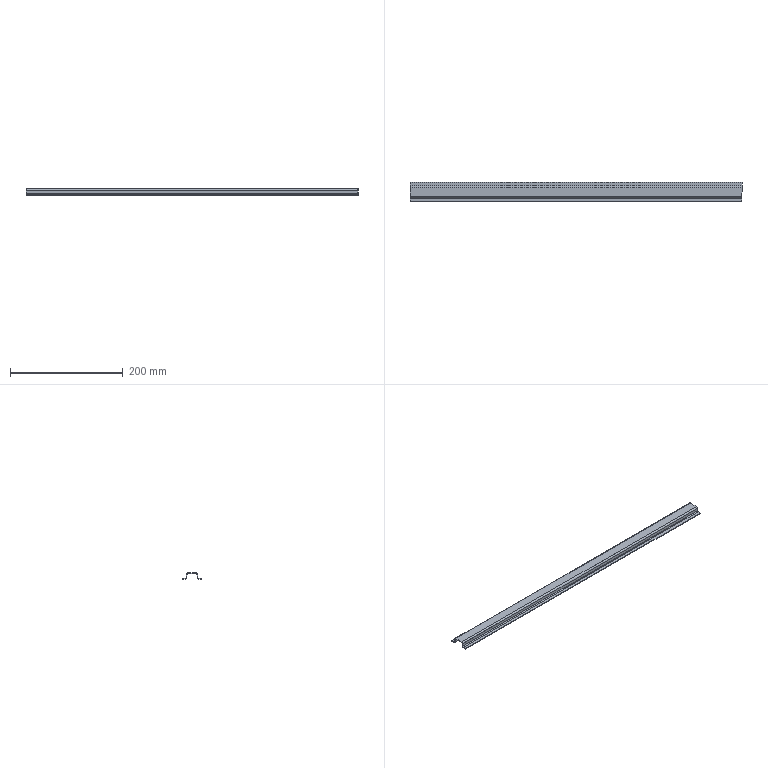Part | SolidWorks | features EdgeFlange 2, FlatPattern 1, SMBaseFlange 1, SheetMetal 1 | 1 solid | 38 faces | box 590 x 34 x 10.7 mm | volume 34971 mm3 | plane 30 | cylinder 8 | commonest cylinder face diameters 3 x4 5.4 x4
STEP:
#1=CARTESIAN_POINT('',(295.,-7.5,0.));
#2=VERTEX_POINT('',#1);
#3=CARTESIAN_POINT('',(295.,7.5,0.));
#4=VERTEX_POINT('',#3);
#5=CARTESIAN_POINT('',(295.,-7.5,0.));
#6=DIRECTION('',(0.,1.,0.));
#7=VECTOR('',#6,1000.);
#8=LINE('',#5,#7);
#9=EDGE_CURVE('',#2,#4,#8,.T.);
#10=ORIENTED_EDGE('',*,*,#9,.F.);
#11=CARTESIAN_POINT('',(295.,-7.5,-1.2));
#12=VERTEX_POINT('',#11);
#13=CARTESIAN_POINT('',(295.,-7.5,-1.2));
#14=DIRECTION('',(0.,0.,1.));
#15=VECTOR('',#14,1000.);
#16=LINE('',#13,#15);
#17=EDGE_CURVE('',#12,#2,#16,.T.);
#18=ORIENTED_EDGE('',*,*,#17,.F.);
#19=CARTESIAN_POINT('',(295.,7.5,-1.2));
#20=VERTEX_POINT('',#19);
#21=CARTESIAN_POINT('',(295.,-7.5,-1.2));
#22=DIRECTION('',(0.,1.,0.));
#23=VECTOR('',#22,1000.);
#24=LINE('',#21,#23);
#25=EDGE_CURVE('',#12,#20,#24,.T.);
#26=ORIENTED_EDGE('',*,*,#25,.T.);
#27=CARTESIAN_POINT('',(295.,7.5,-1.2));
#28=DIRECTION('',(0.,0.,1.));
#29=VECTOR('',#28,1000.);
#30=LINE('',#27,#29);
#31=EDGE_CURVE('',#20,#4,#30,.T.);
#32=ORIENTED_EDGE('',*,*,#31,.T.);
#33=EDGE_LOOP('',(#10,#18,#26,#32));
#34=FACE_OUTER_BOUND('',#33,.T.);
#35=CARTESIAN_POINT('',(295.,-7.5,-1.2));
#36=DIRECTION('',(1.,0.,0.));
#37=DIRECTION('',(0.,0.,-1.));
#38=AXIS2_PLACEMENT_3D('',#35,#36,#37);
#39=PLANE('',#38);
#40=ADVANCED_FACE('',(#34),#39,.T.);
#41=CARTESIAN_POINT('',(-295.,7.5,0.));
#42=VERTEX_POINT('',#41);
#43=CARTESIAN_POINT('',(-295.,-7.5,0.));
#44=VERTEX_POINT('',#43);
#45=CARTESIAN_POINT('',(-295.,-7.5,0.));
#46=DIRECTION('',(0.,-1.,0.));
#47=VECTOR('',#46,1000.);
#48=LINE('',#45,#47);
#49=EDGE_CURVE('',#42,#44,#48,.T.);
#50=ORIENTED_EDGE('',*,*,#49,.F.);
#51=CARTESIAN_POINT('',(-295.,7.5,-1.2));
#52=VERTEX_POINT('',#51);
#53=CARTESIAN_POINT('',(-295.,7.5,-1.2));
#54=DIRECTION('',(0.,0.,1.));
#55=VECTOR('',#54,1000.);
#56=LINE('',#53,#55);
#57=EDGE_CURVE('',#52,#42,#56,.T.);
#58=ORIENTED_EDGE('',*,*,#57,.F.);
#59=CARTESIAN_POINT('',(-295.,-7.5,-1.2));
#60=VERTEX_POINT('',#59);
#61=CARTESIAN_POINT('',(-295.,-7.5,-1.2));
#62=DIRECTION('',(0.,-1.,0.));
#63=VECTOR('',#62,1000.);
#64=LINE('',#61,#63);
#65=EDGE_CURVE('',#52,#60,#64,.T.);
#66=ORIENTED_EDGE('',*,*,#65,.T.);
#67=CARTESIAN_POINT('',(-295.,-7.5,-1.2));
#68=DIRECTION('',(0.,0.,1.));
#69=VECTOR('',#68,1000.);
#70=LINE('',#67,#69);
#71=EDGE_CURVE('',#60,#44,#70,.T.);
#72=ORIENTED_EDGE('',*,*,#71,.T.);
#73=EDGE_LOOP('',(#50,#58,#66,#72));
#74=FACE_OUTER_BOUND('',#73,.T.);
#75=CARTESIAN_POINT('',(-295.,-7.5,-1.2));
#76=DIRECTION('',(-1.,0.,0.));
#77=DIRECTION('',(0.,0.,1.));
#78=AXIS2_PLACEMENT_3D('',#75,#76,#77);
#79=PLANE('',#78);
#80=ADVANCED_FACE('',(#74),#79,.T.);
#81=ORIENTED_EDGE('',*,*,#25,.F.);
#82=CARTESIAN_POINT('',(-295.,-7.5,-1.2));
#83=DIRECTION('',(1.,0.,0.));
#84=VECTOR('',#83,1000.);
#85=LINE('',#82,#84);
#86=EDGE_CURVE('',#60,#12,#85,.T.);
#87=ORIENTED_EDGE('',*,*,#86,.F.);
#88=ORIENTED_EDGE('',*,*,#65,.F.);
#89=CARTESIAN_POINT('',(-295.,7.5,-1.2));
#90=DIRECTION('',(-1.,0.,0.));
#91=VECTOR('',#90,1000.);
#92=LINE('',#89,#91);
#93=EDGE_CURVE('',#20,#52,#92,.T.);
#94=ORIENTED_EDGE('',*,*,#93,.F.);
#95=EDGE_LOOP('',(#81,#87,#88,#94));
#96=FACE_OUTER_BOUND('',#95,.T.);
#97=CARTESIAN_POINT('',(0.,0.,-1.2));
#98=DIRECTION('',(0.,0.,-1.));
#99=DIRECTION('',(-1.,0.,0.));
#100=AXIS2_PLACEMENT_3D('',#97,#98,#99);
#101=PLANE('',#100);
#102=ADVANCED_FACE('',(#96),#101,.T.);
#103=ORIENTED_EDGE('',*,*,#9,.T.);
#104=CARTESIAN_POINT('',(-295.,7.5,0.));
#105=DIRECTION('',(-1.,0.,0.));
#106=VECTOR('',#105,1000.);
#107=LINE('',#104,#106);
#108=EDGE_CURVE('',#4,#42,#107,.T.);
#109=ORIENTED_EDGE('',*,*,#108,.T.);
#110=ORIENTED_EDGE('',*,*,#49,.T.);
#111=CARTESIAN_POINT('',(-295.,-7.5,0.));
#112=DIRECTION('',(1.,0.,0.));
#113=VECTOR('',#112,1000.);
#114=LINE('',#111,#113);
#115=EDGE_CURVE('',#44,#2,#114,.T.);
#116=ORIENTED_EDGE('',*,*,#115,.T.);
#117=EDGE_LOOP('',(#103,#109,#110,#116));
#118=FACE_OUTER_BOUND('',#117,.T.);
#119=CARTESIAN_POINT('',(0.,0.,0.));
#120=DIRECTION('',(0.,0.,-1.));
#121=DIRECTION('',(-1.,0.,0.));
#122=AXIS2_PLACEMENT_3D('',#119,#120,#121);
#123=PLANE('',#122);
#124=ADVANCED_FACE('',(#118),#123,.F.);
#125=CARTESIAN_POINT('',(-295.,9.,-2.7));
#126=VERTEX_POINT('',#125);
#127=CARTESIAN_POINT('',(-295.,10.2,-2.7));
#128=VERTEX_POINT('',#127);
#129=CARTESIAN_POINT('',(-295.,10.2,-2.7));
#130=DIRECTION('',(0.,1.,0.));
#131=VECTOR('',#130,1000.);
#132=LINE('',#129,#131);
#133=EDGE_CURVE('',#126,#128,#132,.T.);
#134=ORIENTED_EDGE('',*,*,#133,.F.);
#135=CARTESIAN_POINT('',(-295.,7.5,-2.7));
#136=DIRECTION('',(-1.,0.,0.));
#137=DIRECTION('',(0.,0.,-1.));
#138=AXIS2_PLACEMENT_3D('',#135,#136,#137);
#139=CIRCLE('',#138,1.5);
#140=EDGE_CURVE('',#52,#126,#139,.T.);
#141=ORIENTED_EDGE('',*,*,#140,.F.);
#142=ORIENTED_EDGE('',*,*,#57,.T.);
#143=CARTESIAN_POINT('',(-295.,7.5,-2.7));
#144=DIRECTION('',(-1.,0.,0.));
#145=DIRECTION('',(0.,0.,-1.));
#146=AXIS2_PLACEMENT_3D('',#143,#144,#145);
#147=CIRCLE('',#146,2.7);
#148=EDGE_CURVE('',#42,#128,#147,.T.);
#149=ORIENTED_EDGE('',*,*,#148,.T.);
#150=EDGE_LOOP('',(#134,#141,#142,#149));
#151=FACE_OUTER_BOUND('',#150,.T.);
#152=CARTESIAN_POINT('',(-295.,7.5,-2.7));
#153=DIRECTION('',(-1.,0.,0.));
#154=DIRECTION('',(0.,0.,1.));
#155=AXIS2_PLACEMENT_3D('',#152,#153,#154);
#156=PLANE('',#155);
#157=ADVANCED_FACE('',(#151),#156,.T.);
#158=CARTESIAN_POINT('',(295.,9.,-2.7));
#159=VERTEX_POINT('',#158);
#160=CARTESIAN_POINT('',(295.,7.5,-2.7));
#161=DIRECTION('',(1.,0.,0.));
#162=DIRECTION('',(0.,0.,-1.));
#163=AXIS2_PLACEMENT_3D('',#160,#161,#162);
#164=CIRCLE('',#163,1.5);
#165=EDGE_CURVE('',#159,#20,#164,.T.);
#166=ORIENTED_EDGE('',*,*,#165,.F.);
#167=CARTESIAN_POINT('',(295.,10.2,-2.7));
#168=VERTEX_POINT('',#167);
#169=CARTESIAN_POINT('',(295.,9.,-2.7));
#170=DIRECTION('',(0.,1.,0.));
#171=VECTOR('',#170,1000.);
#172=LINE('',#169,#171);
#173=EDGE_CURVE('',#159,#168,#172,.T.);
#174=ORIENTED_EDGE('',*,*,#173,.T.);
#175=CARTESIAN_POINT('',(295.,7.5,-2.7));
#176=DIRECTION('',(1.,0.,0.));
#177=DIRECTION('',(0.,0.,-1.));
#178=AXIS2_PLACEMENT_3D('',#175,#176,#177);
#179=CIRCLE('',#178,2.7);
#180=EDGE_CURVE('',#168,#4,#179,.T.);
#181=ORIENTED_EDGE('',*,*,#180,.T.);
#182=ORIENTED_EDGE('',*,*,#31,.F.);
#183=EDGE_LOOP('',(#166,#174,#181,#182));
#184=FACE_OUTER_BOUND('',#183,.T.);
#185=CARTESIAN_POINT('',(295.,7.5,-2.7));
#186=DIRECTION('',(-1.,0.,0.));
#187=DIRECTION('',(0.,0.,1.));
#188=AXIS2_PLACEMENT_3D('',#185,#186,#187);
#189=PLANE('',#188);
#190=ADVANCED_FACE('',(#184),#189,.F.);
#191=ORIENTED_EDGE('',*,*,#108,.F.);
#192=ORIENTED_EDGE('',*,*,#180,.F.);
#193=CARTESIAN_POINT('',(-295.,10.2,-2.7));
#194=DIRECTION('',(-1.,0.,0.));
#195=VECTOR('',#194,1000.);
#196=LINE('',#193,#195);
#197=EDGE_CURVE('',#168,#128,#196,.T.);
#198=ORIENTED_EDGE('',*,*,#197,.T.);
#199=ORIENTED_EDGE('',*,*,#148,.F.);
#200=EDGE_LOOP('',(#191,#192,#198,#199));
#201=FACE_OUTER_BOUND('',#200,.T.);
#202=CARTESIAN_POINT('',(295.,7.5,-2.7));
#203=DIRECTION('',(1.,0.,0.));
#204=DIRECTION('',(0.,1.,0.));
#205=AXIS2_PLACEMENT_3D('',#202,#203,#204);
#206=CYLINDRICAL_SURFACE('',#205,2.7);
#207=ADVANCED_FACE('',(#201),#206,.T.);
#208=ORIENTED_EDGE('',*,*,#93,.T.);
#209=ORIENTED_EDGE('',*,*,#140,.T.);
#210=CARTESIAN_POINT('',(-295.,9.,-2.7));
#211=DIRECTION('',(1.,0.,0.));
#212=VECTOR('',#211,1000.);
#213=LINE('',#210,#212);
#214=EDGE_CURVE('',#126,#159,#213,.T.);
#215=ORIENTED_EDGE('',*,*,#214,.T.);
#216=ORIENTED_EDGE('',*,*,#165,.T.);
#217=EDGE_LOOP('',(#208,#209,#215,#216));
#218=FACE_OUTER_BOUND('',#217,.T.);
#219=CARTESIAN_POINT('',(295.,7.5,-2.7));
#220=DIRECTION('',(1.,0.,0.));
#221=DIRECTION('',(0.,1.,0.));
#222=AXIS2_PLACEMENT_3D('',#219,#220,#221);
#223=CYLINDRICAL_SURFACE('',#222,1.5);
#224=ADVANCED_FACE('',(#218),#223,.F.);
#225=ORIENTED_EDGE('',*,*,#173,.F.);
#226=CARTESIAN_POINT('',(295.,9.,-8.));
#227=VERTEX_POINT('',#226);
#228=CARTESIAN_POINT('',(295.,9.,-8.));
#229=DIRECTION('',(0.,0.,-1.));
#230=VECTOR('',#229,1000.);
#231=LINE('',#228,#230);
#232=EDGE_CURVE('',#159,#227,#231,.T.);
#233=ORIENTED_EDGE('',*,*,#232,.T.);
#234=CARTESIAN_POINT('',(295.,10.2,-8.));
#235=VERTEX_POINT('',#234);
#236=CARTESIAN_POINT('',(295.,10.2,-8.));
#237=DIRECTION('',(0.,-1.,0.));
#238=VECTOR('',#237,1000.);
#239=LINE('',#236,#238);
#240=EDGE_CURVE('',#235,#227,#239,.T.);
#241=ORIENTED_EDGE('',*,*,#240,.F.);
#242=CARTESIAN_POINT('',(295.,10.2,0.));
#243=DIRECTION('',(0.,0.,-1.));
#244=VECTOR('',#243,1000.);
#245=LINE('',#242,#244);
#246=EDGE_CURVE('',#168,#235,#245,.T.);
#247=ORIENTED_EDGE('',*,*,#246,.F.);
#248=EDGE_LOOP('',(#225,#233,#241,#247));
#249=FACE_OUTER_BOUND('',#248,.T.);
#250=CARTESIAN_POINT('',(295.,10.2,-8.));
#251=DIRECTION('',(-1.,0.,0.));
#252=DIRECTION('',(0.,0.,1.));
#253=AXIS2_PLACEMENT_3D('',#250,#251,#252);
#254=PLANE('',#253);
#255=ADVANCED_FACE('',(#249),#254,.F.);
#256=ORIENTED_EDGE('',*,*,#133,.T.);
#257=CARTESIAN_POINT('',(-295.,10.2,-8.));
#258=VERTEX_POINT('',#257);
#259=CARTESIAN_POINT('',(-295.,10.2,0.));
#260=DIRECTION('',(0.,0.,1.));
#261=VECTOR('',#260,1000.);
#262=LINE('',#259,#261);
#263=EDGE_CURVE('',#258,#128,#262,.T.);
#264=ORIENTED_EDGE('',*,*,#263,.F.);
#265=CARTESIAN_POINT('',(-295.,9.,-8.));
#266=VERTEX_POINT('',#265);
#267=CARTESIAN_POINT('',(-295.,10.2,-8.));
#268=DIRECTION('',(0.,-1.,0.));
#269=VECTOR('',#268,1000.);
#270=LINE('',#267,#269);
#271=EDGE_CURVE('',#258,#266,#270,.T.);
#272=ORIENTED_EDGE('',*,*,#271,.T.);
#273=CARTESIAN_POINT('',(-295.,9.,-1.2));
#274=DIRECTION('',(0.,0.,1.));
#275=VECTOR('',#274,1000.);
#276=LINE('',#273,#275);
#277=EDGE_CURVE('',#266,#126,#276,.T.);
#278=ORIENTED_EDGE('',*,*,#277,.T.);
#279=EDGE_LOOP('',(#256,#264,#272,#278));
#280=FACE_OUTER_BOUND('',#279,.T.);
#281=CARTESIAN_POINT('',(-295.,10.2,-1.2));
#282=DIRECTION('',(1.,0.,0.));
#283=DIRECTION('',(0.,0.,-1.));
#284=AXIS2_PLACEMENT_3D('',#281,#282,#283);
#285=PLANE('',#284);
#286=ADVANCED_FACE('',(#280),#285,.F.);
#287=ORIENTED_EDGE('',*,*,#197,.F.);
#288=ORIENTED_EDGE('',*,*,#246,.T.);
#289=CARTESIAN_POINT('',(0.,10.2,-8.));
#290=DIRECTION('',(-1.,0.,0.));
#291=VECTOR('',#290,1000.);
#292=LINE('',#289,#291);
#293=EDGE_CURVE('',#235,#258,#292,.T.);
#294=ORIENTED_EDGE('',*,*,#293,.T.);
#295=ORIENTED_EDGE('',*,*,#263,.T.);
#296=EDGE_LOOP('',(#287,#288,#294,#295));
#297=FACE_OUTER_BOUND('',#296,.T.);
#298=CARTESIAN_POINT('',(0.,10.2,0.));
#299=DIRECTION('',(0.,-1.,0.));
#300=DIRECTION('',(0.,0.,-1.));
#301=AXIS2_PLACEMENT_3D('',#298,#299,#300);
#302=PLANE('',#301);
#303=ADVANCED_FACE('',(#297),#302,.F.);
#304=ORIENTED_EDGE('',*,*,#232,.F.);
#305=ORIENTED_EDGE('',*,*,#214,.F.);
#306=ORIENTED_EDGE('',*,*,#277,.F.);
#307=CARTESIAN_POINT('',(-295.,9.,-8.));
#308=DIRECTION('',(-1.,0.,0.));
#309=VECTOR('',#308,1000.);
#310=LINE('',#307,#309);
#311=EDGE_CURVE('',#227,#266,#310,.T.);
#312=ORIENTED_EDGE('',*,*,#311,.F.);
#313=EDGE_LOOP('',(#304,#305,#306,#312));
#314=FACE_OUTER_BOUND('',#313,.T.);
#315=CARTESIAN_POINT('',(0.,9.,0.));
#316=DIRECTION('',(0.,-1.,0.));
#317=DIRECTION('',(0.,0.,-1.));
#318=AXIS2_PLACEMENT_3D('',#315,#316,#317);
#319=PLANE('',#318);
#320=ADVANCED_FACE('',(#314),#319,.T.);
#321=CARTESIAN_POINT('',(295.,-9.,-2.7));
#322=VERTEX_POINT('',#321);
#323=CARTESIAN_POINT('',(295.,-10.2,-2.7));
#324=VERTEX_POINT('',#323);
#325=CARTESIAN_POINT('',(295.,-10.2,-2.7));
#326=DIRECTION('',(0.,-1.,0.));
#327=VECTOR('',#326,1000.);
#328=LINE('',#325,#327);
#329=EDGE_CURVE('',#322,#324,#328,.T.);
#330=ORIENTED_EDGE('',*,*,#329,.F.);
#331=CARTESIAN_POINT('',(295.,-7.5,-2.7));
#332=DIRECTION('',(1.,0.,0.));
#333=DIRECTION('',(0.,0.,1.));
#334=AXIS2_PLACEMENT_3D('',#331,#332,#333);
#335=CIRCLE('',#334,1.5);
#336=EDGE_CURVE('',#12,#322,#335,.T.);
#337=ORIENTED_EDGE('',*,*,#336,.F.);
#338=ORIENTED_EDGE('',*,*,#17,.T.);
#339=CARTESIAN_POINT('',(295.,-7.5,-2.7));
#340=DIRECTION('',(1.,0.,0.));
#341=DIRECTION('',(0.,0.,1.));
#342=AXIS2_PLACEMENT_3D('',#339,#340,#341);
#343=CIRCLE('',#342,2.7);
#344=EDGE_CURVE('',#2,#324,#343,.T.);
#345=ORIENTED_EDGE('',*,*,#344,.T.);
#346=EDGE_LOOP('',(#330,#337,#338,#345));
#347=FACE_OUTER_BOUND('',#346,.T.);
#348=CARTESIAN_POINT('',(295.,-7.5,-2.7));
#349=DIRECTION('',(1.,0.,0.));
#350=DIRECTION('',(0.,0.,-1.));
#351=AXIS2_PLACEMENT_3D('',#348,#349,#350);
#352=PLANE('',#351);
#353=ADVANCED_FACE('',(#347),#352,.T.);
#354=CARTESIAN_POINT('',(-295.,-9.,-2.7));
#355=VERTEX_POINT('',#354);
#356=CARTESIAN_POINT('',(-295.,-7.5,-2.7));
#357=DIRECTION('',(-1.,0.,0.));
#358=DIRECTION('',(0.,0.,1.));
#359=AXIS2_PLACEMENT_3D('',#356,#357,#358);
#360=CIRCLE('',#359,1.5);
#361=EDGE_CURVE('',#355,#60,#360,.T.);
#362=ORIENTED_EDGE('',*,*,#361,.F.);
#363=CARTESIAN_POINT('',(-295.,-10.2,-2.7));
#364=VERTEX_POINT('',#363);
#365=CARTESIAN_POINT('',(-295.,-9.,-2.7));
#366=DIRECTION('',(0.,-1.,0.));
#367=VECTOR('',#366,1000.);
#368=LINE('',#365,#367);
#369=EDGE_CURVE('',#355,#364,#368,.T.);
#370=ORIENTED_EDGE('',*,*,#369,.T.);
#371=CARTESIAN_POINT('',(-295.,-7.5,-2.7));
#372=DIRECTION('',(-1.,0.,0.));
#373=DIRECTION('',(0.,0.,1.));
#374=AXIS2_PLACEMENT_3D('',#371,#372,#373);
#375=CIRCLE('',#374,2.7);
#376=EDGE_CURVE('',#364,#44,#375,.T.);
#377=ORIENTED_EDGE('',*,*,#376,.T.);
#378=ORIENTED_EDGE('',*,*,#71,.F.);
#379=EDGE_LOOP('',(#362,#370,#377,#378));
#380=FACE_OUTER_BOUND('',#379,.T.);
#381=CARTESIAN_POINT('',(-295.,-7.5,-2.7));
#382=DIRECTION('',(1.,0.,0.));
#383=DIRECTION('',(0.,0.,-1.));
#384=AXIS2_PLACEMENT_3D('',#381,#382,#383);
#385=PLANE('',#384);
#386=ADVANCED_FACE('',(#380),#385,.F.);
#387=ORIENTED_EDGE('',*,*,#115,.F.);
#388=ORIENTED_EDGE('',*,*,#376,.F.);
#389=CARTESIAN_POINT('',(295.,-10.2,-2.7));
#390=DIRECTION('',(1.,0.,0.));
#391=VECTOR('',#390,1000.);
#392=LINE('',#389,#391);
#393=EDGE_CURVE('',#364,#324,#392,.T.);
#394=ORIENTED_EDGE('',*,*,#393,.T.);
#395=ORIENTED_EDGE('',*,*,#344,.F.);
#396=EDGE_LOOP('',(#387,#388,#394,#395));
#397=FACE_OUTER_BOUND('',#396,.T.);
#398=CARTESIAN_POINT('',(-295.,-7.5,-2.7));
#399=DIRECTION('',(-1.,0.,0.));
#400=DIRECTION('',(0.,-1.,0.));
#401=AXIS2_PLACEMENT_3D('',#398,#399,#400);
#402=CYLINDRICAL_SURFACE('',#401,2.7);
#403=ADVANCED_FACE('',(#397),#402,.T.);
#404=ORIENTED_EDGE('',*,*,#86,.T.);
#405=ORIENTED_EDGE('',*,*,#336,.T.);
#406=CARTESIAN_POINT('',(295.,-9.,-2.7));
#407=DIRECTION('',(-1.,0.,0.));
#408=VECTOR('',#407,1000.);
#409=LINE('',#406,#408);
#410=EDGE_CURVE('',#322,#355,#409,.T.);
#411=ORIENTED_EDGE('',*,*,#410,.T.);
#412=ORIENTED_EDGE('',*,*,#361,.T.);
#413=EDGE_LOOP('',(#404,#405,#411,#412));
#414=FACE_OUTER_BOUND('',#413,.T.);
#415=CARTESIAN_POINT('',(-295.,-7.5,-2.7));
#416=DIRECTION('',(-1.,0.,0.));
#417=DIRECTION('',(0.,-1.,0.));
#418=AXIS2_PLACEMENT_3D('',#415,#416,#417);
#419=CYLINDRICAL_SURFACE('',#418,1.5);
#420=ADVANCED_FACE('',(#414),#419,.F.);
#421=ORIENTED_EDGE('',*,*,#369,.F.);
#422=CARTESIAN_POINT('',(-295.,-9.,-8.));
#423=VERTEX_POINT('',#422);
#424=CARTESIAN_POINT('',(-295.,-9.,-8.));
#425=DIRECTION('',(0.,0.,-1.));
#426=VECTOR('',#425,1000.);
#427=LINE('',#424,#426);
#428=EDGE_CURVE('',#355,#423,#427,.T.);
#429=ORIENTED_EDGE('',*,*,#428,.T.);
#430=CARTESIAN_POINT('',(-295.,-10.2,-8.));
#431=VERTEX_POINT('',#430);
#432=CARTESIAN_POINT('',(-295.,-10.2,-8.));
#433=DIRECTION('',(0.,1.,0.));
#434=VECTOR('',#433,1000.);
#435=LINE('',#432,#434);
#436=EDGE_CURVE('',#431,#423,#435,.T.);
#437=ORIENTED_EDGE('',*,*,#436,.F.);
#438=CARTESIAN_POINT('',(-295.,-10.2,0.));
#439=DIRECTION('',(0.,0.,-1.));
#440=VECTOR('',#439,1000.);
#441=LINE('',#438,#440);
#442=EDGE_CURVE('',#364,#431,#441,.T.);
#443=ORIENTED_EDGE('',*,*,#442,.F.);
#444=EDGE_LOOP('',(#421,#429,#437,#443));
#445=FACE_OUTER_BOUND('',#444,.T.);
#446=CARTESIAN_POINT('',(-295.,-10.2,-8.));
#447=DIRECTION('',(1.,0.,0.));
#448=DIRECTION('',(0.,0.,-1.));
#449=AXIS2_PLACEMENT_3D('',#446,#447,#448);
#450=PLANE('',#449);
#451=ADVANCED_FACE('',(#445),#450,.F.);
#452=ORIENTED_EDGE('',*,*,#329,.T.);
#453=CARTESIAN_POINT('',(295.,-10.2,-8.));
#454=VERTEX_POINT('',#453);
#455=CARTESIAN_POINT('',(295.,-10.2,0.));
#456=DIRECTION('',(0.,0.,1.));
#457=VECTOR('',#456,1000.);
#458=LINE('',#455,#457);
#459=EDGE_CURVE('',#454,#324,#458,.T.);
#460=ORIENTED_EDGE('',*,*,#459,.F.);
#461=CARTESIAN_POINT('',(295.,-9.,-8.));
#462=VERTEX_POINT('',#461);
#463=CARTESIAN_POINT('',(295.,-10.2,-8.));
#464=DIRECTION('',(0.,1.,0.));
#465=VECTOR('',#464,1000.);
#466=LINE('',#463,#465);
#467=EDGE_CURVE('',#454,#462,#466,.T.);
#468=ORIENTED_EDGE('',*,*,#467,.T.);
#469=CARTESIAN_POINT('',(295.,-9.,-1.2));
#470=DIRECTION('',(0.,0.,1.));
#471=VECTOR('',#470,1000.);
#472=LINE('',#469,#471);
#473=EDGE_CURVE('',#462,#322,#472,.T.);
#474=ORIENTED_EDGE('',*,*,#473,.T.);
#475=EDGE_LOOP('',(#452,#460,#468,#474));
#476=FACE_OUTER_BOUND('',#475,.T.);
#477=CARTESIAN_POINT('',(295.,-10.2,-1.2));
#478=DIRECTION('',(-1.,0.,0.));
#479=DIRECTION('',(0.,0.,1.));
#480=AXIS2_PLACEMENT_3D('',#477,#478,#479);
#481=PLANE('',#480);
#482=ADVANCED_FACE('',(#476),#481,.F.);
#483=ORIENTED_EDGE('',*,*,#393,.F.);
#484=ORIENTED_EDGE('',*,*,#442,.T.);
#485=CARTESIAN_POINT('',(0.,-10.2,-8.));
#486=DIRECTION('',(1.,0.,0.));
#487=VECTOR('',#486,1000.);
#488=LINE('',#485,#487);
#489=EDGE_CURVE('',#431,#454,#488,.T.);
#490=ORIENTED_EDGE('',*,*,#489,.T.);
#491=ORIENTED_EDGE('',*,*,#459,.T.);
#492=EDGE_LOOP('',(#483,#484,#490,#491));
#493=FACE_OUTER_BOUND('',#492,.T.);
#494=CARTESIAN_POINT('',(0.,-10.2,0.));
#495=DIRECTION('',(0.,1.,0.));
#496=DIRECTION('',(0.,0.,1.));
#497=AXIS2_PLACEMENT_3D('',#494,#495,#496);
#498=PLANE('',#497);
#499=ADVANCED_FACE('',(#493),#498,.F.);
#500=ORIENTED_EDGE('',*,*,#428,.F.);
#501=ORIENTED_EDGE('',*,*,#410,.F.);
#502=ORIENTED_EDGE('',*,*,#473,.F.);
#503=CARTESIAN_POINT('',(295.,-9.,-8.));
#504=DIRECTION('',(1.,0.,0.));
#505=VECTOR('',#504,1000.);
#506=LINE('',#503,#505);
#507=EDGE_CURVE('',#423,#462,#506,.T.);
#508=ORIENTED_EDGE('',*,*,#507,.F.);
#509=EDGE_LOOP('',(#500,#501,#502,#508));
#510=FACE_OUTER_BOUND('',#509,.T.);
#511=CARTESIAN_POINT('',(0.,-9.,0.));
#512=DIRECTION('',(0.,1.,0.));
#513=DIRECTION('',(0.,0.,1.));
#514=AXIS2_PLACEMENT_3D('',#511,#512,#513);
#515=PLANE('',#514);
#516=ADVANCED_FACE('',(#510),#515,.T.);
#517=CARTESIAN_POINT('',(295.,11.7,-9.5));
#518=VERTEX_POINT('',#517);
#519=CARTESIAN_POINT('',(295.,11.7,-10.7));
#520=VERTEX_POINT('',#519);
#521=CARTESIAN_POINT('',(295.,11.7,-10.7));
#522=DIRECTION('',(0.,0.,-1.));
#523=VECTOR('',#522,1000.);
#524=LINE('',#521,#523);
#525=EDGE_CURVE('',#518,#520,#524,.T.);
#526=ORIENTED_EDGE('',*,*,#525,.F.);
#527=CARTESIAN_POINT('',(295.,11.7,-8.));
#528=DIRECTION('',(1.,0.,0.));
#529=DIRECTION('',(0.,0.,1.));
#530=AXIS2_PLACEMENT_3D('',#527,#528,#529);
#531=CIRCLE('',#530,1.5);
#532=EDGE_CURVE('',#235,#518,#531,.T.);
#533=ORIENTED_EDGE('',*,*,#532,.F.);
#534=ORIENTED_EDGE('',*,*,#240,.T.);
#535=CARTESIAN_POINT('',(295.,11.7,-8.));
#536=DIRECTION('',(1.,0.,0.));
#537=DIRECTION('',(0.,0.,1.));
#538=AXIS2_PLACEMENT_3D('',#535,#536,#537);
#539=CIRCLE('',#538,2.7);
#540=EDGE_CURVE('',#227,#520,#539,.T.);
#541=ORIENTED_EDGE('',*,*,#540,.T.);
#542=EDGE_LOOP('',(#526,#533,#534,#541));
#543=FACE_OUTER_BOUND('',#542,.T.);
#544=CARTESIAN_POINT('',(295.,11.7,-8.));
#545=DIRECTION('',(1.,0.,0.));
#546=DIRECTION('',(0.,0.,-1.));
#547=AXIS2_PLACEMENT_3D('',#544,#545,#546);
#548=PLANE('',#547);
#549=ADVANCED_FACE('',(#543),#548,.T.);
#550=CARTESIAN_POINT('',(-295.,11.7,-9.5));
#551=VERTEX_POINT('',#550);
#552=CARTESIAN_POINT('',(-295.,11.7,-8.));
#553=DIRECTION('',(-1.,0.,0.));
#554=DIRECTION('',(0.,0.,1.));
#555=AXIS2_PLACEMENT_3D('',#552,#553,#554);
#556=CIRCLE('',#555,1.5);
#557=EDGE_CURVE('',#551,#258,#556,.T.);
#558=ORIENTED_EDGE('',*,*,#557,.F.);
#559=CARTESIAN_POINT('',(-295.,11.7,-10.7));
#560=VERTEX_POINT('',#559);
#561=CARTESIAN_POINT('',(-295.,11.7,-9.5));
#562=DIRECTION('',(0.,0.,-1.));
#563=VECTOR('',#562,1000.);
#564=LINE('',#561,#563);
#565=EDGE_CURVE('',#551,#560,#564,.T.);
#566=ORIENTED_EDGE('',*,*,#565,.T.);
#567=CARTESIAN_POINT('',(-295.,11.7,-8.));
#568=DIRECTION('',(-1.,0.,0.));
#569=DIRECTION('',(0.,0.,1.));
#570=AXIS2_PLACEMENT_3D('',#567,#568,#569);
#571=CIRCLE('',#570,2.7);
#572=EDGE_CURVE('',#560,#266,#571,.T.);
#573=ORIENTED_EDGE('',*,*,#572,.T.);
#574=ORIENTED_EDGE('',*,*,#271,.F.);
#575=EDGE_LOOP('',(#558,#566,#573,#574));
#576=FACE_OUTER_BOUND('',#575,.T.);
#577=CARTESIAN_POINT('',(-295.,11.7,-8.));
#578=DIRECTION('',(1.,0.,0.));
#579=DIRECTION('',(0.,0.,-1.));
#580=AXIS2_PLACEMENT_3D('',#577,#578,#579);
#581=PLANE('',#580);
#582=ADVANCED_FACE('',(#576),#581,.F.);
#583=ORIENTED_EDGE('',*,*,#311,.T.);
#584=ORIENTED_EDGE('',*,*,#572,.F.);
#585=CARTESIAN_POINT('',(0.,11.7,-10.7));
#586=DIRECTION('',(-1.,0.,0.));
#587=VECTOR('',#586,1000.);
#588=LINE('',#585,#587);
#589=EDGE_CURVE('',#520,#560,#588,.T.);
#590=ORIENTED_EDGE('',*,*,#589,.F.);
#591=ORIENTED_EDGE('',*,*,#540,.F.);
#592=EDGE_LOOP('',(#583,#584,#590,#591));
#593=FACE_OUTER_BOUND('',#592,.T.);
#594=CARTESIAN_POINT('',(-295.,11.7,-8.));
#595=DIRECTION('',(-1.,0.,0.));
#596=DIRECTION('',(0.,0.,-1.));
#597=AXIS2_PLACEMENT_3D('',#594,#595,#596);
#598=CYLINDRICAL_SURFACE('',#597,2.7);
#599=ADVANCED_FACE('',(#593),#598,.T.);
#600=ORIENTED_EDGE('',*,*,#293,.F.);
#601=ORIENTED_EDGE('',*,*,#532,.T.);
#602=CARTESIAN_POINT('',(295.,11.7,-9.5));
#603=DIRECTION('',(-1.,0.,0.));
#604=VECTOR('',#603,1000.);
#605=LINE('',#602,#604);
#606=EDGE_CURVE('',#518,#551,#605,.T.);
#607=ORIENTED_EDGE('',*,*,#606,.T.);
#608=ORIENTED_EDGE('',*,*,#557,.T.);
#609=EDGE_LOOP('',(#600,#601,#607,#608));
#610=FACE_OUTER_BOUND('',#609,.T.);
#611=CARTESIAN_POINT('',(-295.,11.7,-8.));
#612=DIRECTION('',(-1.,0.,0.));
#613=DIRECTION('',(0.,0.,-1.));
#614=AXIS2_PLACEMENT_3D('',#611,#612,#613);
#615=CYLINDRICAL_SURFACE('',#614,1.5);
#616=ADVANCED_FACE('',(#610),#615,.F.);
#617=CARTESIAN_POINT('',(-295.,17.,-10.7));
#618=VERTEX_POINT('',#617);
#619=CARTESIAN_POINT('',(-295.,10.2,-10.7));
#620=DIRECTION('',(0.,-1.,0.));
#621=VECTOR('',#620,1000.);
#622=LINE('',#619,#621);
#623=EDGE_CURVE('',#618,#560,#622,.T.);
#624=ORIENTED_EDGE('',*,*,#623,.T.);
#625=ORIENTED_EDGE('',*,*,#565,.F.);
#626=CARTESIAN_POINT('',(-295.,17.,-9.5));
#627=VERTEX_POINT('',#626);
#628=CARTESIAN_POINT('',(-295.,0.,-9.5));
#629=DIRECTION('',(0.,-1.,0.));
#630=VECTOR('',#629,1000.);
#631=LINE('',#628,#630);
#632=EDGE_CURVE('',#627,#551,#631,.T.);
#633=ORIENTED_EDGE('',*,*,#632,.F.);
#634=CARTESIAN_POINT('',(-295.,17.,-10.7));
#635=DIRECTION('',(0.,0.,1.));
#636=VECTOR('',#635,1000.);
#637=LINE('',#634,#636);
#638=EDGE_CURVE('',#618,#627,#637,.T.);
#639=ORIENTED_EDGE('',*,*,#638,.F.);
#640=EDGE_LOOP('',(#624,#625,#633,#639));
#641=FACE_OUTER_BOUND('',#640,.T.);
#642=CARTESIAN_POINT('',(-295.,10.2,-10.7));
#643=DIRECTION('',(-1.,0.,0.));
#644=DIRECTION('',(0.,0.,1.));
#645=AXIS2_PLACEMENT_3D('',#642,#643,#644);
#646=PLANE('',#645);
#647=ADVANCED_FACE('',(#641),#646,.T.);
#648=CARTESIAN_POINT('',(295.,17.,-9.5));
#649=VERTEX_POINT('',#648);
#650=CARTESIAN_POINT('',(295.,0.,-9.5));
#651=DIRECTION('',(0.,1.,0.));
#652=VECTOR('',#651,1000.);
#653=LINE('',#650,#652);
#654=EDGE_CURVE('',#518,#649,#653,.T.);
#655=ORIENTED_EDGE('',*,*,#654,.F.);
#656=ORIENTED_EDGE('',*,*,#525,.T.);
#657=CARTESIAN_POINT('',(295.,17.,-10.7));
#658=VERTEX_POINT('',#657);
#659=CARTESIAN_POINT('',(295.,17.,-10.7));
#660=DIRECTION('',(0.,1.,0.));
#661=VECTOR('',#660,1000.);
#662=LINE('',#659,#661);
#663=EDGE_CURVE('',#520,#658,#662,.T.);
#664=ORIENTED_EDGE('',*,*,#663,.T.);
#665=CARTESIAN_POINT('',(295.,17.,-10.7));
#666=DIRECTION('',(0.,0.,1.));
#667=VECTOR('',#666,1000.);
#668=LINE('',#665,#667);
#669=EDGE_CURVE('',#658,#649,#668,.T.);
#670=ORIENTED_EDGE('',*,*,#669,.T.);
#671=EDGE_LOOP('',(#655,#656,#664,#670));
#672=FACE_OUTER_BOUND('',#671,.T.);
#673=CARTESIAN_POINT('',(295.,17.,-10.7));
#674=DIRECTION('',(1.,0.,0.));
#675=DIRECTION('',(0.,1.,0.));
#676=AXIS2_PLACEMENT_3D('',#673,#674,#675);
#677=PLANE('',#676);
#678=ADVANCED_FACE('',(#672),#677,.T.);
#679=ORIENTED_EDGE('',*,*,#663,.F.);
#680=ORIENTED_EDGE('',*,*,#589,.T.);
#681=ORIENTED_EDGE('',*,*,#623,.F.);
#682=CARTESIAN_POINT('',(-295.,17.,-10.7));
#683=DIRECTION('',(-1.,0.,0.));
#684=VECTOR('',#683,1000.);
#685=LINE('',#682,#684);
#686=EDGE_CURVE('',#658,#618,#685,.T.);
#687=ORIENTED_EDGE('',*,*,#686,.F.);
#688=EDGE_LOOP('',(#679,#680,#681,#687));
#689=FACE_OUTER_BOUND('',#688,.T.);
#690=CARTESIAN_POINT('',(0.,0.,-10.7));
#691=DIRECTION('',(0.,0.,-1.));
#692=DIRECTION('',(-1.,0.,0.));
#693=AXIS2_PLACEMENT_3D('',#690,#691,#692);
#694=PLANE('',#693);
#695=ADVANCED_FACE('',(#689),#694,.T.);
#696=ORIENTED_EDGE('',*,*,#606,.F.);
#697=ORIENTED_EDGE('',*,*,#654,.T.);
#698=CARTESIAN_POINT('',(0.,17.,-9.5));
#699=DIRECTION('',(-1.,0.,0.));
#700=VECTOR('',#699,1000.);
#701=LINE('',#698,#700);
#702=EDGE_CURVE('',#649,#627,#701,.T.);
#703=ORIENTED_EDGE('',*,*,#702,.T.);
#704=ORIENTED_EDGE('',*,*,#632,.T.);
#705=EDGE_LOOP('',(#696,#697,#703,#704));
#706=FACE_OUTER_BOUND('',#705,.T.);
#707=CARTESIAN_POINT('',(0.,0.,-9.5));
#708=DIRECTION('',(0.,0.,-1.));
#709=DIRECTION('',(-1.,0.,0.));
#710=AXIS2_PLACEMENT_3D('',#707,#708,#709);
#711=PLANE('',#710);
#712=ADVANCED_FACE('',(#706),#711,.F.);
#713=ORIENTED_EDGE('',*,*,#702,.F.);
#714=ORIENTED_EDGE('',*,*,#669,.F.);
#715=ORIENTED_EDGE('',*,*,#686,.T.);
#716=ORIENTED_EDGE('',*,*,#638,.T.);
#717=EDGE_LOOP('',(#713,#714,#715,#716));
#718=FACE_OUTER_BOUND('',#717,.T.);
#719=CARTESIAN_POINT('',(-295.,17.,-10.7));
#720=DIRECTION('',(0.,1.,0.));
#721=DIRECTION('',(0.,0.,1.));
#722=AXIS2_PLACEMENT_3D('',#719,#720,#721);
#723=PLANE('',#722);
#724=ADVANCED_FACE('',(#718),#723,.T.);
#725=CARTESIAN_POINT('',(-295.,-11.7,-9.5));
#726=VERTEX_POINT('',#725);
#727=CARTESIAN_POINT('',(-295.,-11.7,-10.7));
#728=VERTEX_POINT('',#727);
#729=CARTESIAN_POINT('',(-295.,-11.7,-10.7));
#730=DIRECTION('',(0.,0.,-1.));
#731=VECTOR('',#730,1000.);
#732=LINE('',#729,#731);
#733=EDGE_CURVE('',#726,#728,#732,.T.);
#734=ORIENTED_EDGE('',*,*,#733,.F.);
#735=CARTESIAN_POINT('',(-295.,-11.7,-8.));
#736=DIRECTION('',(-1.,0.,0.));
#737=DIRECTION('',(0.,0.,-1.));
#738=AXIS2_PLACEMENT_3D('',#735,#736,#737);
#739=CIRCLE('',#738,1.5);
#740=EDGE_CURVE('',#431,#726,#739,.T.);
#741=ORIENTED_EDGE('',*,*,#740,.F.);
#742=ORIENTED_EDGE('',*,*,#436,.T.);
#743=CARTESIAN_POINT('',(-295.,-11.7,-8.));
#744=DIRECTION('',(-1.,0.,0.));
#745=DIRECTION('',(0.,0.,-1.));
#746=AXIS2_PLACEMENT_3D('',#743,#744,#745);
#747=CIRCLE('',#746,2.7);
#748=EDGE_CURVE('',#423,#728,#747,.T.);
#749=ORIENTED_EDGE('',*,*,#748,.T.);
#750=EDGE_LOOP('',(#734,#741,#742,#749));
#751=FACE_OUTER_BOUND('',#750,.T.);
#752=CARTESIAN_POINT('',(-295.,-11.7,-8.));
#753=DIRECTION('',(-1.,0.,0.));
#754=DIRECTION('',(0.,0.,1.));
#755=AXIS2_PLACEMENT_3D('',#752,#753,#754);
#756=PLANE('',#755);
#757=ADVANCED_FACE('',(#751),#756,.T.);
#758=CARTESIAN_POINT('',(295.,-11.7,-9.5));
#759=VERTEX_POINT('',#758);
#760=CARTESIAN_POINT('',(295.,-11.7,-8.));
#761=DIRECTION('',(1.,0.,0.));
#762=DIRECTION('',(0.,0.,-1.));
#763=AXIS2_PLACEMENT_3D('',#760,#761,#762);
#764=CIRCLE('',#763,1.5);
#765=EDGE_CURVE('',#759,#454,#764,.T.);
#766=ORIENTED_EDGE('',*,*,#765,.F.);
#767=CARTESIAN_POINT('',(295.,-11.7,-10.7));
#768=VERTEX_POINT('',#767);
#769=CARTESIAN_POINT('',(295.,-11.7,-9.5));
#770=DIRECTION('',(0.,0.,-1.));
#771=VECTOR('',#770,1000.);
#772=LINE('',#769,#771);
#773=EDGE_CURVE('',#759,#768,#772,.T.);
#774=ORIENTED_EDGE('',*,*,#773,.T.);
#775=CARTESIAN_POINT('',(295.,-11.7,-8.));
#776=DIRECTION('',(1.,0.,0.));
#777=DIRECTION('',(0.,0.,-1.));
#778=AXIS2_PLACEMENT_3D('',#775,#776,#777);
#779=CIRCLE('',#778,2.7);
#780=EDGE_CURVE('',#768,#462,#779,.T.);
#781=ORIENTED_EDGE('',*,*,#780,.T.);
#782=ORIENTED_EDGE('',*,*,#467,.F.);
#783=EDGE_LOOP('',(#766,#774,#781,#782));
#784=FACE_OUTER_BOUND('',#783,.T.);
#785=CARTESIAN_POINT('',(295.,-11.7,-8.));
#786=DIRECTION('',(-1.,0.,0.));
#787=DIRECTION('',(0.,0.,1.));
#788=AXIS2_PLACEMENT_3D('',#785,#786,#787);
#789=PLANE('',#788);
#790=ADVANCED_FACE('',(#784),#789,.F.);
#791=ORIENTED_EDGE('',*,*,#507,.T.);
#792=ORIENTED_EDGE('',*,*,#780,.F.);
#793=CARTESIAN_POINT('',(-295.,-11.7,-10.7));
#794=DIRECTION('',(-1.,0.,0.));
#795=VECTOR('',#794,1000.);
#796=LINE('',#793,#795);
#797=EDGE_CURVE('',#768,#728,#796,.T.);
#798=ORIENTED_EDGE('',*,*,#797,.T.);
#799=ORIENTED_EDGE('',*,*,#748,.F.);
#800=EDGE_LOOP('',(#791,#792,#798,#799));
#801=FACE_OUTER_BOUND('',#800,.T.);
#802=CARTESIAN_POINT('',(295.,-11.7,-8.));
#803=DIRECTION('',(1.,0.,0.));
#804=DIRECTION('',(0.,0.,-1.));
#805=AXIS2_PLACEMENT_3D('',#802,#803,#804);
#806=CYLINDRICAL_SURFACE('',#805,2.7);
#807=ADVANCED_FACE('',(#801),#806,.T.);
#808=ORIENTED_EDGE('',*,*,#489,.F.);
#809=ORIENTED_EDGE('',*,*,#740,.T.);
#810=CARTESIAN_POINT('',(-295.,-11.7,-9.5));
#811=DIRECTION('',(1.,0.,0.));
#812=VECTOR('',#811,1000.);
#813=LINE('',#810,#812);
#814=EDGE_CURVE('',#726,#759,#813,.T.);
#815=ORIENTED_EDGE('',*,*,#814,.T.);
#816=ORIENTED_EDGE('',*,*,#765,.T.);
#817=EDGE_LOOP('',(#808,#809,#815,#816));
#818=FACE_OUTER_BOUND('',#817,.T.);
#819=CARTESIAN_POINT('',(295.,-11.7,-8.));
#820=DIRECTION('',(1.,0.,0.));
#821=DIRECTION('',(0.,0.,-1.));
#822=AXIS2_PLACEMENT_3D('',#819,#820,#821);
#823=CYLINDRICAL_SURFACE('',#822,1.5);
#824=ADVANCED_FACE('',(#818),#823,.F.);
#825=CARTESIAN_POINT('',(-295.,-17.,-9.5));
#826=VERTEX_POINT('',#825);
#827=CARTESIAN_POINT('',(-295.,0.,-9.5));
#828=DIRECTION('',(0.,-1.,0.));
#829=VECTOR('',#828,1000.);
#830=LINE('',#827,#829);
#831=EDGE_CURVE('',#726,#826,#830,.T.);
#832=ORIENTED_EDGE('',*,*,#831,.F.);
#833=ORIENTED_EDGE('',*,*,#733,.T.);
#834=CARTESIAN_POINT('',(-295.,-17.,-10.7));
#835=VERTEX_POINT('',#834);
#836=CARTESIAN_POINT('',(-295.,-10.2,-10.7));
#837=DIRECTION('',(0.,-1.,0.));
#838=VECTOR('',#837,1000.);
#839=LINE('',#836,#838);
#840=EDGE_CURVE('',#728,#835,#839,.T.);
#841=ORIENTED_EDGE('',*,*,#840,.T.);
#842=CARTESIAN_POINT('',(-295.,-17.,-10.7));
#843=DIRECTION('',(0.,0.,1.));
#844=VECTOR('',#843,1000.);
#845=LINE('',#842,#844);
#846=EDGE_CURVE('',#835,#826,#845,.T.);
#847=ORIENTED_EDGE('',*,*,#846,.T.);
#848=EDGE_LOOP('',(#832,#833,#841,#847));
#849=FACE_OUTER_BOUND('',#848,.T.);
#850=CARTESIAN_POINT('',(-295.,-10.2,-10.7));
#851=DIRECTION('',(-1.,0.,0.));
#852=DIRECTION('',(0.,0.,1.));
#853=AXIS2_PLACEMENT_3D('',#850,#851,#852);
#854=PLANE('',#853);
#855=ADVANCED_FACE('',(#849),#854,.T.);
#856=CARTESIAN_POINT('',(295.,-17.,-10.7));
#857=VERTEX_POINT('',#856);
#858=CARTESIAN_POINT('',(295.,-17.,-10.7));
#859=DIRECTION('',(0.,1.,0.));
#860=VECTOR('',#859,1000.);
#861=LINE('',#858,#860);
#862=EDGE_CURVE('',#857,#768,#861,.T.);
#863=ORIENTED_EDGE('',*,*,#862,.T.);
#864=ORIENTED_EDGE('',*,*,#773,.F.);
#865=CARTESIAN_POINT('',(295.,-17.,-9.5));
#866=VERTEX_POINT('',#865);
#867=CARTESIAN_POINT('',(295.,0.,-9.5));
#868=DIRECTION('',(0.,1.,0.));
#869=VECTOR('',#868,1000.);
#870=LINE('',#867,#869);
#871=EDGE_CURVE('',#866,#759,#870,.T.);
#872=ORIENTED_EDGE('',*,*,#871,.F.);
#873=CARTESIAN_POINT('',(295.,-17.,-10.7));
#874=DIRECTION('',(0.,0.,1.));
#875=VECTOR('',#874,1000.);
#876=LINE('',#873,#875);
#877=EDGE_CURVE('',#857,#866,#876,.T.);
#878=ORIENTED_EDGE('',*,*,#877,.F.);
#879=EDGE_LOOP('',(#863,#864,#872,#878));
#880=FACE_OUTER_BOUND('',#879,.T.);
#881=CARTESIAN_POINT('',(295.,-17.,-10.7));
#882=DIRECTION('',(1.,0.,0.));
#883=DIRECTION('',(0.,1.,0.));
#884=AXIS2_PLACEMENT_3D('',#881,#882,#883);
#885=PLANE('',#884);
#886=ADVANCED_FACE('',(#880),#885,.T.);
#887=ORIENTED_EDGE('',*,*,#797,.F.);
#888=ORIENTED_EDGE('',*,*,#862,.F.);
#889=CARTESIAN_POINT('',(-295.,-17.,-10.7));
#890=DIRECTION('',(1.,0.,0.));
#891=VECTOR('',#890,1000.);
#892=LINE('',#889,#891);
#893=EDGE_CURVE('',#835,#857,#892,.T.);
#894=ORIENTED_EDGE('',*,*,#893,.F.);
#895=ORIENTED_EDGE('',*,*,#840,.F.);
#896=EDGE_LOOP('',(#887,#888,#894,#895));
#897=FACE_OUTER_BOUND('',#896,.T.);
#898=CARTESIAN_POINT('',(0.,0.,-10.7));
#899=DIRECTION('',(0.,0.,1.));
#900=DIRECTION('',(1.,0.,0.));
#901=AXIS2_PLACEMENT_3D('',#898,#899,#900);
#902=PLANE('',#901);
#903=ADVANCED_FACE('',(#897),#902,.F.);
#904=ORIENTED_EDGE('',*,*,#871,.T.);
#905=ORIENTED_EDGE('',*,*,#814,.F.);
#906=ORIENTED_EDGE('',*,*,#831,.T.);
#907=CARTESIAN_POINT('',(0.,-17.,-9.5));
#908=DIRECTION('',(1.,0.,0.));
#909=VECTOR('',#908,1000.);
#910=LINE('',#907,#909);
#911=EDGE_CURVE('',#826,#866,#910,.T.);
#912=ORIENTED_EDGE('',*,*,#911,.T.);
#913=EDGE_LOOP('',(#904,#905,#906,#912));
#914=FACE_OUTER_BOUND('',#913,.T.);
#915=CARTESIAN_POINT('',(0.,0.,-9.5));
#916=DIRECTION('',(0.,0.,1.));
#917=DIRECTION('',(1.,0.,0.));
#918=AXIS2_PLACEMENT_3D('',#915,#916,#917);
#919=PLANE('',#918);
#920=ADVANCED_FACE('',(#914),#919,.T.);
#921=ORIENTED_EDGE('',*,*,#911,.F.);
#922=ORIENTED_EDGE('',*,*,#846,.F.);
#923=ORIENTED_EDGE('',*,*,#893,.T.);
#924=ORIENTED_EDGE('',*,*,#877,.T.);
#925=EDGE_LOOP('',(#921,#922,#923,#924));
#926=FACE_OUTER_BOUND('',#925,.T.);
#927=CARTESIAN_POINT('',(-295.,-17.,-10.7));
#928=DIRECTION('',(0.,-1.,0.));
#929=DIRECTION('',(1.,0.,0.));
#930=AXIS2_PLACEMENT_3D('',#927,#928,#929);
#931=PLANE('',#930);
#932=ADVANCED_FACE('',(#926),#931,.T.);
#933=CLOSED_SHELL('',(#40,#80,#102,#124,#157,#190,#207,#224,#255,#286,#303,#320,#353,#386,#403,#420,#451,#482,#499,#516,#549,#582,#599,#616,#647,#678,#695,#712,#724,#757,#790,#807,#824,#855,#886,#903,#920,#932));
#934=MANIFOLD_SOLID_BREP('',#933);
#935=CARTESIAN_POINT('',(0.,0.,0.));
#936=DIRECTION('',(0.,0.,1.));
#937=DIRECTION('',(1.,0.,0.));
#938=AXIS2_PLACEMENT_3D('',#935,#936,#937);
#939=(LENGTH_UNIT()NAMED_UNIT(*)SI_UNIT(.MILLI.,.METRE.));
#940=UNCERTAINTY_MEASURE_WITH_UNIT(LENGTH_MEASURE(0.00001),#939,'','');
#941=(NAMED_UNIT(*)PLANE_ANGLE_UNIT()SI_UNIT($,.RADIAN.));
#942=(NAMED_UNIT(*)SI_UNIT($,.STERADIAN.)SOLID_ANGLE_UNIT());
#943=(GEOMETRIC_REPRESENTATION_CONTEXT(3)GLOBAL_UNCERTAINTY_ASSIGNED_CONTEXT((#940))GLOBAL_UNIT_ASSIGNED_CONTEXT((#939,#941,#942))REPRESENTATION_CONTEXT('',''));
#944=ADVANCED_BREP_SHAPE_REPRESENTATION('',(#934,#938),#943);